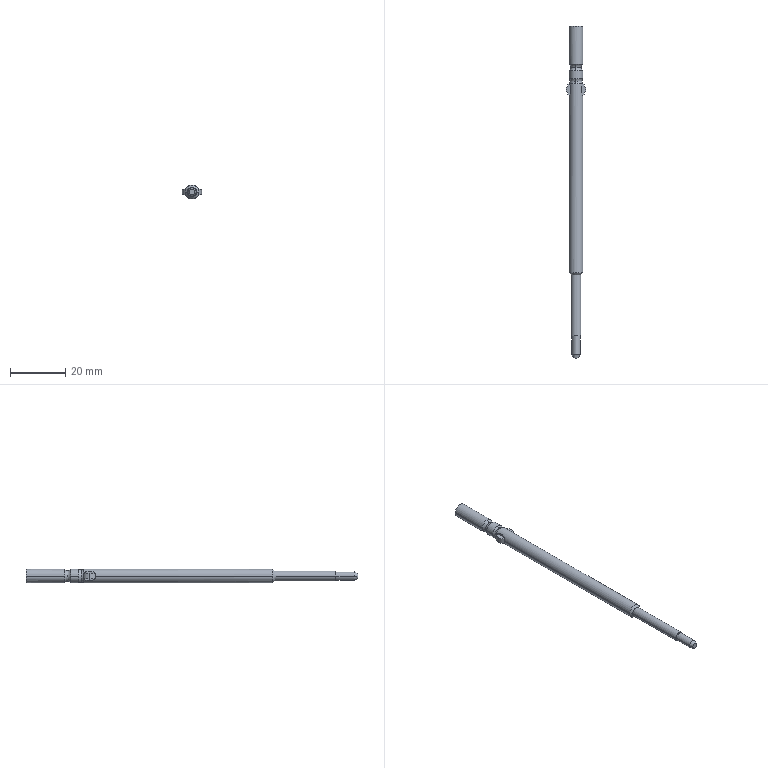Part | SolidWorks | features MoveFace 6, ICE 4, Chamfer 1, MirrorPattern 1, RevCut 1, Revolution 1 | 1 solid | 46 faces | box 7 x 120 x 5 mm | volume 2019 mm3 | cylinder 19 | plane 15 | torus 8 | cone 4 | commonest cylinder face diameters 5 x6 9.339 x6 5.269 x3 2.983 x2 3.5 x2
STEP:
#1=CARTESIAN_POINT('',(0.,116.2,2.5));
#2=VERTEX_POINT('',#1);
#3=CARTESIAN_POINT('',(0.,115.,1.9));
#4=VERTEX_POINT('',#3);
#5=CARTESIAN_POINT('',(0.,115.,3.4));
#6=DIRECTION('',(-1.,0.,0.));
#7=DIRECTION('',(0.,0.,1.));
#8=AXIS2_PLACEMENT_3D('',#5,#6,#7);
#9=CIRCLE('',#8,1.5);
#10=EDGE_CURVE('',#2,#4,#9,.T.);
#11=ORIENTED_EDGE('',*,*,#10,.T.);
#12=CARTESIAN_POINT('',(0.,115.,-1.9));
#13=VERTEX_POINT('',#12);
#14=CARTESIAN_POINT('',(0.,115.,0.));
#15=DIRECTION('',(0.,1.,0.));
#16=DIRECTION('',(0.,0.,1.));
#17=AXIS2_PLACEMENT_3D('',#14,#15,#16);
#18=CIRCLE('',#17,1.9);
#19=EDGE_CURVE('',#4,#13,#18,.T.);
#20=ORIENTED_EDGE('',*,*,#19,.T.);
#21=CARTESIAN_POINT('',(0.,116.2,-2.5));
#22=VERTEX_POINT('',#21);
#23=CARTESIAN_POINT('',(0.,115.,-3.4));
#24=DIRECTION('',(1.,0.,0.));
#25=DIRECTION('',(0.,0.,-1.));
#26=AXIS2_PLACEMENT_3D('',#23,#24,#25);
#27=CIRCLE('',#26,1.5);
#28=EDGE_CURVE('',#22,#13,#27,.T.);
#29=ORIENTED_EDGE('',*,*,#28,.F.);
#30=CARTESIAN_POINT('',(2.5,116.2,0.));
#31=VERTEX_POINT('',#30);
#32=CARTESIAN_POINT('',(0.,116.2,0.));
#33=DIRECTION('',(0.,-1.,0.));
#34=DIRECTION('',(0.,0.,-1.));
#35=AXIS2_PLACEMENT_3D('',#32,#33,#34);
#36=CIRCLE('',#35,2.5);
#37=EDGE_CURVE('',#22,#31,#36,.T.);
#38=ORIENTED_EDGE('',*,*,#37,.T.);
#39=CARTESIAN_POINT('',(0.,116.2,0.));
#40=DIRECTION('',(0.,-1.,0.));
#41=DIRECTION('',(0.,0.,-1.));
#42=AXIS2_PLACEMENT_3D('',#39,#40,#41);
#43=CIRCLE('',#42,2.5);
#44=EDGE_CURVE('',#31,#2,#43,.T.);
#45=ORIENTED_EDGE('',*,*,#44,.T.);
#46=EDGE_LOOP('',(#11,#20,#29,#38,#45));
#47=FACE_OUTER_BOUND('',#46,.T.);
#48=CARTESIAN_POINT('',(0.,115.,0.));
#49=DIRECTION('',(0.,1.,0.));
#50=DIRECTION('',(0.,0.,1.));
#51=AXIS2_PLACEMENT_3D('',#48,#49,#50);
#52=TOROIDAL_SURFACE('',#51,3.4,1.5);
#53=ADVANCED_FACE('',(#47),#52,.F.);
#54=CARTESIAN_POINT('',(0.,110.867,2.5));
#55=VERTEX_POINT('',#54);
#56=CARTESIAN_POINT('',(0.,110.,2.15));
#57=VERTEX_POINT('',#56);
#58=CARTESIAN_POINT('',(0.,110.,3.4));
#59=DIRECTION('',(-1.,0.,0.));
#60=DIRECTION('',(0.,0.,1.));
#61=AXIS2_PLACEMENT_3D('',#58,#59,#60);
#62=CIRCLE('',#61,1.25);
#63=EDGE_CURVE('',#55,#57,#62,.T.);
#64=ORIENTED_EDGE('',*,*,#63,.T.);
#65=CARTESIAN_POINT('',(0.,110.,-2.15));
#66=VERTEX_POINT('',#65);
#67=CARTESIAN_POINT('',(0.,110.,0.));
#68=DIRECTION('',(0.,1.,0.));
#69=DIRECTION('',(0.,0.,1.));
#70=AXIS2_PLACEMENT_3D('',#67,#68,#69);
#71=CIRCLE('',#70,2.15);
#72=EDGE_CURVE('',#57,#66,#71,.T.);
#73=ORIENTED_EDGE('',*,*,#72,.T.);
#74=CARTESIAN_POINT('',(0.,110.867,-2.5));
#75=VERTEX_POINT('',#74);
#76=CARTESIAN_POINT('',(0.,110.,-3.4));
#77=DIRECTION('',(1.,0.,0.));
#78=DIRECTION('',(0.,0.,-1.));
#79=AXIS2_PLACEMENT_3D('',#76,#77,#78);
#80=CIRCLE('',#79,1.25);
#81=EDGE_CURVE('',#75,#66,#80,.T.);
#82=ORIENTED_EDGE('',*,*,#81,.F.);
#83=CARTESIAN_POINT('',(2.5,110.867,0.));
#84=VERTEX_POINT('',#83);
#85=CARTESIAN_POINT('',(0.,110.867,0.));
#86=DIRECTION('',(0.,-1.,0.));
#87=DIRECTION('',(0.,0.,-1.));
#88=AXIS2_PLACEMENT_3D('',#85,#86,#87);
#89=CIRCLE('',#88,2.5);
#90=EDGE_CURVE('',#75,#84,#89,.T.);
#91=ORIENTED_EDGE('',*,*,#90,.T.);
#92=CARTESIAN_POINT('',(0.,110.867,0.));
#93=DIRECTION('',(0.,-1.,0.));
#94=DIRECTION('',(0.,0.,-1.));
#95=AXIS2_PLACEMENT_3D('',#92,#93,#94);
#96=CIRCLE('',#95,2.5);
#97=EDGE_CURVE('',#84,#55,#96,.T.);
#98=ORIENTED_EDGE('',*,*,#97,.T.);
#99=EDGE_LOOP('',(#64,#73,#82,#91,#98));
#100=FACE_OUTER_BOUND('',#99,.T.);
#101=CARTESIAN_POINT('',(0.,110.,0.));
#102=DIRECTION('',(0.,1.,0.));
#103=DIRECTION('',(0.,0.,1.));
#104=AXIS2_PLACEMENT_3D('',#101,#102,#103);
#105=TOROIDAL_SURFACE('',#104,3.4,1.25);
#106=ADVANCED_FACE('',(#100),#105,.F.);
#107=ORIENTED_EDGE('',*,*,#81,.T.);
#108=CARTESIAN_POINT('',(0.,110.,0.));
#109=DIRECTION('',(0.,1.,0.));
#110=DIRECTION('',(0.,0.,1.));
#111=AXIS2_PLACEMENT_3D('',#108,#109,#110);
#112=CIRCLE('',#111,2.15);
#113=EDGE_CURVE('',#66,#57,#112,.T.);
#114=ORIENTED_EDGE('',*,*,#113,.T.);
#115=ORIENTED_EDGE('',*,*,#63,.F.);
#116=CARTESIAN_POINT('',(-2.5,110.867,0.));
#117=VERTEX_POINT('',#116);
#118=CARTESIAN_POINT('',(0.,110.867,0.));
#119=DIRECTION('',(0.,-1.,0.));
#120=DIRECTION('',(0.,0.,-1.));
#121=AXIS2_PLACEMENT_3D('',#118,#119,#120);
#122=CIRCLE('',#121,2.5);
#123=EDGE_CURVE('',#55,#117,#122,.T.);
#124=ORIENTED_EDGE('',*,*,#123,.T.);
#125=CARTESIAN_POINT('',(0.,110.867,0.));
#126=DIRECTION('',(0.,-1.,0.));
#127=DIRECTION('',(0.,0.,-1.));
#128=AXIS2_PLACEMENT_3D('',#125,#126,#127);
#129=CIRCLE('',#128,2.5);
#130=EDGE_CURVE('',#117,#75,#129,.T.);
#131=ORIENTED_EDGE('',*,*,#130,.T.);
#132=EDGE_LOOP('',(#107,#114,#115,#124,#131));
#133=FACE_OUTER_BOUND('',#132,.T.);
#134=CARTESIAN_POINT('',(0.,110.,0.));
#135=DIRECTION('',(0.,1.,0.));
#136=DIRECTION('',(0.,0.,1.));
#137=AXIS2_PLACEMENT_3D('',#134,#135,#136);
#138=TOROIDAL_SURFACE('',#137,3.4,1.25);
#139=ADVANCED_FACE('',(#133),#138,.F.);
#140=ORIENTED_EDGE('',*,*,#28,.T.);
#141=CARTESIAN_POINT('',(0.,115.,0.));
#142=DIRECTION('',(0.,1.,0.));
#143=DIRECTION('',(0.,0.,1.));
#144=AXIS2_PLACEMENT_3D('',#141,#142,#143);
#145=CIRCLE('',#144,1.9);
#146=EDGE_CURVE('',#13,#4,#145,.T.);
#147=ORIENTED_EDGE('',*,*,#146,.T.);
#148=ORIENTED_EDGE('',*,*,#10,.F.);
#149=CARTESIAN_POINT('',(-2.5,116.2,0.));
#150=VERTEX_POINT('',#149);
#151=CARTESIAN_POINT('',(0.,116.2,0.));
#152=DIRECTION('',(0.,-1.,0.));
#153=DIRECTION('',(0.,0.,-1.));
#154=AXIS2_PLACEMENT_3D('',#151,#152,#153);
#155=CIRCLE('',#154,2.5);
#156=EDGE_CURVE('',#2,#150,#155,.T.);
#157=ORIENTED_EDGE('',*,*,#156,.T.);
#158=CARTESIAN_POINT('',(0.,116.2,0.));
#159=DIRECTION('',(0.,-1.,0.));
#160=DIRECTION('',(0.,0.,-1.));
#161=AXIS2_PLACEMENT_3D('',#158,#159,#160);
#162=CIRCLE('',#161,2.5);
#163=EDGE_CURVE('',#150,#22,#162,.T.);
#164=ORIENTED_EDGE('',*,*,#163,.T.);
#165=EDGE_LOOP('',(#140,#147,#148,#157,#164));
#166=FACE_OUTER_BOUND('',#165,.T.);
#167=CARTESIAN_POINT('',(0.,115.,0.));
#168=DIRECTION('',(0.,1.,0.));
#169=DIRECTION('',(0.,0.,1.));
#170=AXIS2_PLACEMENT_3D('',#167,#168,#169);
#171=TOROIDAL_SURFACE('',#170,3.4,1.5);
#172=ADVANCED_FACE('',(#166),#171,.F.);
#173=CARTESIAN_POINT('',(-1.75,40.,0.));
#174=VERTEX_POINT('',#173);
#175=CARTESIAN_POINT('',(1.75,40.,0.));
#176=VERTEX_POINT('',#175);
#177=CARTESIAN_POINT('',(0.,40.,0.));
#178=DIRECTION('',(0.,1.,0.));
#179=DIRECTION('',(-1.,0.,0.));
#180=AXIS2_PLACEMENT_3D('',#177,#178,#179);
#181=CIRCLE('',#180,1.75);
#182=EDGE_CURVE('',#174,#176,#181,.T.);
#183=ORIENTED_EDGE('',*,*,#182,.T.);
#184=CARTESIAN_POINT('',(2.5,40.75,0.));
#185=VERTEX_POINT('',#184);
#186=CARTESIAN_POINT('',(2.5,40.75,0.));
#187=DIRECTION('',(0.7071,0.7071,0.));
#188=VECTOR('',#187,1000.);
#189=LINE('',#186,#188);
#190=EDGE_CURVE('',#176,#185,#189,.T.);
#191=ORIENTED_EDGE('',*,*,#190,.T.);
#192=CARTESIAN_POINT('',(-2.5,40.75,0.));
#193=VERTEX_POINT('',#192);
#194=CARTESIAN_POINT('',(0.,40.75,0.));
#195=DIRECTION('',(0.,1.,0.));
#196=DIRECTION('',(-1.,0.,0.));
#197=AXIS2_PLACEMENT_3D('',#194,#195,#196);
#198=CIRCLE('',#197,2.5);
#199=EDGE_CURVE('',#193,#185,#198,.T.);
#200=ORIENTED_EDGE('',*,*,#199,.F.);
#201=CARTESIAN_POINT('',(-2.5,40.75,0.));
#202=DIRECTION('',(-0.7071,0.7071,0.));
#203=VECTOR('',#202,1000.);
#204=LINE('',#201,#203);
#205=EDGE_CURVE('',#174,#193,#204,.T.);
#206=ORIENTED_EDGE('',*,*,#205,.F.);
#207=EDGE_LOOP('',(#183,#191,#200,#206));
#208=FACE_OUTER_BOUND('',#207,.T.);
#209=CARTESIAN_POINT('',(0.,40.75,0.));
#210=DIRECTION('',(0.,1.,0.));
#211=DIRECTION('',(-1.,0.,0.));
#212=AXIS2_PLACEMENT_3D('',#209,#210,#211);
#213=CONICAL_SURFACE('',#212,2.5,0.7854);
#214=ADVANCED_FACE('',(#208),#213,.T.);
#215=CARTESIAN_POINT('',(-1.017,10.,0.));
#216=VERTEX_POINT('',#215);
#217=CARTESIAN_POINT('',(1.017,10.,0.));
#218=VERTEX_POINT('',#217);
#219=CARTESIAN_POINT('',(0.,10.,0.));
#220=DIRECTION('',(0.,1.,0.));
#221=DIRECTION('',(-1.,0.,0.));
#222=AXIS2_PLACEMENT_3D('',#219,#220,#221);
#223=CIRCLE('',#222,1.017);
#224=EDGE_CURVE('',#216,#218,#223,.T.);
#225=ORIENTED_EDGE('',*,*,#224,.T.);
#226=CARTESIAN_POINT('',(1.491,11.265,0.));
#227=VERTEX_POINT('',#226);
#228=CARTESIAN_POINT('',(0.9841,9.912,0.));
#229=DIRECTION('',(0.3511,0.9363,0.));
#230=VECTOR('',#229,1000.);
#231=LINE('',#228,#230);
#232=EDGE_CURVE('',#218,#227,#231,.T.);
#233=ORIENTED_EDGE('',*,*,#232,.T.);
#234=CARTESIAN_POINT('',(-1.491,11.265,0.));
#235=VERTEX_POINT('',#234);
#236=CARTESIAN_POINT('',(0.,11.265,0.));
#237=DIRECTION('',(0.,1.,0.));
#238=DIRECTION('',(-1.,0.,0.));
#239=AXIS2_PLACEMENT_3D('',#236,#237,#238);
#240=CIRCLE('',#239,1.491);
#241=EDGE_CURVE('',#235,#227,#240,.T.);
#242=ORIENTED_EDGE('',*,*,#241,.F.);
#243=CARTESIAN_POINT('',(-0.9841,9.912,0.));
#244=DIRECTION('',(-0.3511,0.9363,0.));
#245=VECTOR('',#244,1000.);
#246=LINE('',#243,#245);
#247=EDGE_CURVE('',#216,#235,#246,.T.);
#248=ORIENTED_EDGE('',*,*,#247,.F.);
#249=EDGE_LOOP('',(#225,#233,#242,#248));
#250=FACE_OUTER_BOUND('',#249,.T.);
#251=CARTESIAN_POINT('',(0.,9.912,0.));
#252=DIRECTION('',(0.,1.,0.));
#253=DIRECTION('',(-1.,0.,0.));
#254=AXIS2_PLACEMENT_3D('',#251,#252,#253);
#255=CONICAL_SURFACE('',#254,0.9841,0.3588);
#256=ADVANCED_FACE('',(#250),#255,.T.);
#257=CARTESIAN_POINT('',(1.491,18.,0.));
#258=VERTEX_POINT('',#257);
#259=CARTESIAN_POINT('',(-1.491,18.,0.));
#260=VERTEX_POINT('',#259);
#261=CARTESIAN_POINT('',(0.,18.,0.));
#262=DIRECTION('',(0.,-1.,0.));
#263=DIRECTION('',(1.,0.,0.));
#264=AXIS2_PLACEMENT_3D('',#261,#262,#263);
#265=CIRCLE('',#264,1.491);
#266=EDGE_CURVE('',#258,#260,#265,.T.);
#267=ORIENTED_EDGE('',*,*,#266,.T.);
#268=CARTESIAN_POINT('',(-1.491,8.,0.));
#269=DIRECTION('',(0.,-1.,0.));
#270=VECTOR('',#269,1000.);
#271=LINE('',#268,#270);
#272=EDGE_CURVE('',#260,#235,#271,.T.);
#273=ORIENTED_EDGE('',*,*,#272,.T.);
#274=ORIENTED_EDGE('',*,*,#241,.T.);
#275=CARTESIAN_POINT('',(1.491,8.,0.));
#276=DIRECTION('',(0.,-1.,0.));
#277=VECTOR('',#276,1000.);
#278=LINE('',#275,#277);
#279=EDGE_CURVE('',#258,#227,#278,.T.);
#280=ORIENTED_EDGE('',*,*,#279,.F.);
#281=EDGE_LOOP('',(#267,#273,#274,#280));
#282=FACE_OUTER_BOUND('',#281,.T.);
#283=CARTESIAN_POINT('',(0.,8.,0.));
#284=DIRECTION('',(0.,-1.,0.));
#285=DIRECTION('',(1.,0.,0.));
#286=AXIS2_PLACEMENT_3D('',#283,#284,#285);
#287=CYLINDRICAL_SURFACE('',#286,1.491);
#288=ADVANCED_FACE('',(#282),#287,.T.);
#289=CARTESIAN_POINT('',(-1.809,107.066,-1.725));
#290=VERTEX_POINT('',#289);
#291=CARTESIAN_POINT('',(-2.291,109.133,-1.));
#292=VERTEX_POINT('',#291);
#293=CARTESIAN_POINT('',(-1.809,107.066,-1.725));
#294=CARTESIAN_POINT('',(-1.809,107.454,-1.725));
#295=CARTESIAN_POINT('',(-1.858,107.835,-1.679));
#296=CARTESIAN_POINT('',(-1.993,108.376,-1.511));
#297=CARTESIAN_POINT('',(-2.047,108.547,-1.44));
#298=CARTESIAN_POINT('',(-2.166,108.864,-1.254));
#299=CARTESIAN_POINT('',(-2.231,109.01,-1.139));
#300=CARTESIAN_POINT('',(-2.291,109.133,-1.));
#301=B_SPLINE_CURVE_WITH_KNOTS('',3,(#293,#294,#295,#296,#297,#298,#299,#300),.UNSPECIFIED.,.F.,.F.,(4,2,2,4),(0.01141,0.01257,0.01314,0.01372),.UNSPECIFIED.);
#302=EDGE_CURVE('',#290,#292,#301,.T.);
#303=ORIENTED_EDGE('',*,*,#302,.F.);
#304=CARTESIAN_POINT('',(-1.809,107.066,-1.));
#305=VERTEX_POINT('',#304);
#306=CARTESIAN_POINT('',(-1.809,107.066,-4.));
#307=DIRECTION('',(0.,0.,1.));
#308=VECTOR('',#307,1000.);
#309=LINE('',#306,#308);
#310=EDGE_CURVE('',#290,#305,#309,.T.);
#311=ORIENTED_EDGE('',*,*,#310,.T.);
#312=CARTESIAN_POINT('',(-6.479,107.066,-1.));
#313=DIRECTION('',(0.,0.,1.));
#314=DIRECTION('',(-1.,0.,0.));
#315=AXIS2_PLACEMENT_3D('',#312,#313,#314);
#316=CIRCLE('',#315,4.669);
#317=EDGE_CURVE('',#305,#292,#316,.T.);
#318=ORIENTED_EDGE('',*,*,#317,.T.);
#319=EDGE_LOOP('',(#303,#311,#318));
#320=FACE_OUTER_BOUND('',#319,.T.);
#321=CARTESIAN_POINT('',(-6.479,107.066,-4.));
#322=DIRECTION('',(0.,0.,1.));
#323=DIRECTION('',(1.,0.,0.));
#324=AXIS2_PLACEMENT_3D('',#321,#322,#323);
#325=CYLINDRICAL_SURFACE('',#324,4.669);
#326=ADVANCED_FACE('',(#320),#325,.F.);
#327=CARTESIAN_POINT('',(2.291,109.133,1.));
#328=VERTEX_POINT('',#327);
#329=CARTESIAN_POINT('',(1.809,107.066,1.725));
#330=VERTEX_POINT('',#329);
#331=CARTESIAN_POINT('',(2.291,109.133,1.));
#332=CARTESIAN_POINT('',(2.231,109.009,1.139));
#333=CARTESIAN_POINT('',(2.167,108.867,1.252));
#334=CARTESIAN_POINT('',(2.047,108.548,1.439));
#335=CARTESIAN_POINT('',(1.993,108.377,1.511));
#336=CARTESIAN_POINT('',(1.904,108.02,1.622));
#337=CARTESIAN_POINT('',(1.868,107.831,1.661));
#338=CARTESIAN_POINT('',(1.821,107.452,1.713));
#339=CARTESIAN_POINT('',(1.809,107.26,1.725));
#340=CARTESIAN_POINT('',(1.809,107.066,1.725));
#341=B_SPLINE_CURVE_WITH_KNOTS('',3,(#331,#332,#333,#334,#335,#336,#337,#338,#339,#340),.UNSPECIFIED.,.F.,.F.,(4,2,2,2,4),(0.009093,0.009672,0.01025,0.01083,0.01141),.UNSPECIFIED.);
#342=EDGE_CURVE('',#328,#330,#341,.T.);
#343=ORIENTED_EDGE('',*,*,#342,.T.);
#344=CARTESIAN_POINT('',(1.809,107.066,1.));
#345=VERTEX_POINT('',#344);
#346=CARTESIAN_POINT('',(1.809,107.066,4.));
#347=DIRECTION('',(0.,0.,-1.));
#348=VECTOR('',#347,1000.);
#349=LINE('',#346,#348);
#350=EDGE_CURVE('',#330,#345,#349,.T.);
#351=ORIENTED_EDGE('',*,*,#350,.T.);
#352=CARTESIAN_POINT('',(6.479,107.066,1.));
#353=DIRECTION('',(0.,0.,1.));
#354=DIRECTION('',(1.,0.,0.));
#355=AXIS2_PLACEMENT_3D('',#352,#353,#354);
#356=CIRCLE('',#355,4.669);
#357=EDGE_CURVE('',#328,#345,#356,.T.);
#358=ORIENTED_EDGE('',*,*,#357,.F.);
#359=EDGE_LOOP('',(#343,#351,#358));
#360=FACE_OUTER_BOUND('',#359,.T.);
#361=CARTESIAN_POINT('',(6.479,107.066,4.));
#362=DIRECTION('',(0.,0.,-1.));
#363=DIRECTION('',(-1.,0.,0.));
#364=AXIS2_PLACEMENT_3D('',#361,#362,#363);
#365=CYLINDRICAL_SURFACE('',#364,4.669);
#366=ADVANCED_FACE('',(#360),#365,.F.);
#367=CARTESIAN_POINT('',(-3.5,107.066,1.));
#368=VERTEX_POINT('',#367);
#369=CARTESIAN_POINT('',(-2.5,105.,1.));
#370=VERTEX_POINT('',#369);
#371=CARTESIAN_POINT('',(-0.8653,107.066,1.));
#372=DIRECTION('',(0.,0.,1.));
#373=DIRECTION('',(1.,0.,0.));
#374=AXIS2_PLACEMENT_3D('',#371,#372,#373);
#375=CIRCLE('',#374,2.635);
#376=EDGE_CURVE('',#368,#370,#375,.T.);
#377=ORIENTED_EDGE('',*,*,#376,.F.);
#378=CARTESIAN_POINT('',(-3.5,107.066,-1.));
#379=VERTEX_POINT('',#378);
#380=CARTESIAN_POINT('',(-3.5,107.066,1.));
#381=DIRECTION('',(0.,0.,-1.));
#382=VECTOR('',#381,1000.);
#383=LINE('',#380,#382);
#384=EDGE_CURVE('',#368,#379,#383,.T.);
#385=ORIENTED_EDGE('',*,*,#384,.T.);
#386=CARTESIAN_POINT('',(-2.5,105.,-1.));
#387=VERTEX_POINT('',#386);
#388=CARTESIAN_POINT('',(-0.8653,107.066,-1.));
#389=DIRECTION('',(0.,0.,1.));
#390=DIRECTION('',(1.,0.,0.));
#391=AXIS2_PLACEMENT_3D('',#388,#389,#390);
#392=CIRCLE('',#391,2.635);
#393=EDGE_CURVE('',#379,#387,#392,.T.);
#394=ORIENTED_EDGE('',*,*,#393,.T.);
#395=CARTESIAN_POINT('',(-2.5,105.,0.));
#396=VERTEX_POINT('',#395);
#397=CARTESIAN_POINT('',(-2.5,105.,1.));
#398=DIRECTION('',(0.,0.,-1.));
#399=VECTOR('',#398,1000.);
#400=LINE('',#397,#399);
#401=EDGE_CURVE('',#396,#387,#400,.T.);
#402=ORIENTED_EDGE('',*,*,#401,.F.);
#403=CARTESIAN_POINT('',(-2.5,105.,1.));
#404=DIRECTION('',(0.,0.,-1.));
#405=VECTOR('',#404,1000.);
#406=LINE('',#403,#405);
#407=EDGE_CURVE('',#370,#396,#406,.T.);
#408=ORIENTED_EDGE('',*,*,#407,.F.);
#409=EDGE_LOOP('',(#377,#385,#394,#402,#408));
#410=FACE_OUTER_BOUND('',#409,.T.);
#411=CARTESIAN_POINT('',(-0.8653,107.066,1.));
#412=DIRECTION('',(0.,0.,-1.));
#413=DIRECTION('',(-1.,0.,0.));
#414=AXIS2_PLACEMENT_3D('',#411,#412,#413);
#415=CYLINDRICAL_SURFACE('',#414,2.635);
#416=ADVANCED_FACE('',(#410),#415,.T.);
#417=ORIENTED_EDGE('',*,*,#97,.F.);
#418=CARTESIAN_POINT('',(2.5,113.8,0.));
#419=VERTEX_POINT('',#418);
#420=CARTESIAN_POINT('',(2.5,120.,0.));
#421=DIRECTION('',(0.,1.,0.));
#422=VECTOR('',#421,1000.);
#423=LINE('',#420,#422);
#424=EDGE_CURVE('',#84,#419,#423,.T.);
#425=ORIENTED_EDGE('',*,*,#424,.T.);
#426=CARTESIAN_POINT('',(0.,113.8,2.5));
#427=VERTEX_POINT('',#426);
#428=CARTESIAN_POINT('',(0.,113.8,0.));
#429=DIRECTION('',(0.,1.,0.));
#430=DIRECTION('',(0.,0.,1.));
#431=AXIS2_PLACEMENT_3D('',#428,#429,#430);
#432=CIRCLE('',#431,2.5);
#433=EDGE_CURVE('',#427,#419,#432,.T.);
#434=ORIENTED_EDGE('',*,*,#433,.F.);
#435=CARTESIAN_POINT('',(-2.5,113.8,0.));
#436=VERTEX_POINT('',#435);
#437=CARTESIAN_POINT('',(0.,113.8,0.));
#438=DIRECTION('',(0.,1.,0.));
#439=DIRECTION('',(0.,0.,1.));
#440=AXIS2_PLACEMENT_3D('',#437,#438,#439);
#441=CIRCLE('',#440,2.5);
#442=EDGE_CURVE('',#436,#427,#441,.T.);
#443=ORIENTED_EDGE('',*,*,#442,.F.);
#444=CARTESIAN_POINT('',(-2.5,120.,0.));
#445=DIRECTION('',(0.,1.,0.));
#446=VECTOR('',#445,1000.);
#447=LINE('',#444,#446);
#448=EDGE_CURVE('',#117,#436,#447,.T.);
#449=ORIENTED_EDGE('',*,*,#448,.F.);
#450=ORIENTED_EDGE('',*,*,#123,.F.);
#451=EDGE_LOOP('',(#417,#425,#434,#443,#449,#450));
#452=FACE_OUTER_BOUND('',#451,.T.);
#453=CARTESIAN_POINT('',(0.,120.,0.));
#454=DIRECTION('',(0.,1.,0.));
#455=DIRECTION('',(-1.,0.,0.));
#456=AXIS2_PLACEMENT_3D('',#453,#454,#455);
#457=CYLINDRICAL_SURFACE('',#456,2.5);
#458=ADVANCED_FACE('',(#452),#457,.T.);
#459=ORIENTED_EDGE('',*,*,#146,.F.);
#460=CARTESIAN_POINT('',(0.,113.8,-2.5));
#461=VERTEX_POINT('',#460);
#462=CARTESIAN_POINT('',(0.,115.,-3.4));
#463=DIRECTION('',(1.,0.,0.));
#464=DIRECTION('',(0.,0.,-1.));
#465=AXIS2_PLACEMENT_3D('',#462,#463,#464);
#466=CIRCLE('',#465,1.5);
#467=EDGE_CURVE('',#13,#461,#466,.T.);
#468=ORIENTED_EDGE('',*,*,#467,.T.);
#469=CARTESIAN_POINT('',(0.,113.8,0.));
#470=DIRECTION('',(0.,1.,0.));
#471=DIRECTION('',(0.,0.,1.));
#472=AXIS2_PLACEMENT_3D('',#469,#470,#471);
#473=CIRCLE('',#472,2.5);
#474=EDGE_CURVE('',#461,#436,#473,.T.);
#475=ORIENTED_EDGE('',*,*,#474,.T.);
#476=ORIENTED_EDGE('',*,*,#442,.T.);
#477=CARTESIAN_POINT('',(0.,115.,3.4));
#478=DIRECTION('',(-1.,0.,0.));
#479=DIRECTION('',(0.,0.,1.));
#480=AXIS2_PLACEMENT_3D('',#477,#478,#479);
#481=CIRCLE('',#480,1.5);
#482=EDGE_CURVE('',#4,#427,#481,.T.);
#483=ORIENTED_EDGE('',*,*,#482,.F.);
#484=EDGE_LOOP('',(#459,#468,#475,#476,#483));
#485=FACE_OUTER_BOUND('',#484,.T.);
#486=CARTESIAN_POINT('',(0.,115.,0.));
#487=DIRECTION('',(0.,1.,0.));
#488=DIRECTION('',(0.,0.,1.));
#489=AXIS2_PLACEMENT_3D('',#486,#487,#488);
#490=TOROIDAL_SURFACE('',#489,3.4,1.5);
#491=ADVANCED_FACE('',(#485),#490,.F.);
#492=ORIENTED_EDGE('',*,*,#44,.F.);
#493=CARTESIAN_POINT('',(2.5,130.,0.));
#494=VERTEX_POINT('',#493);
#495=CARTESIAN_POINT('',(2.5,120.,0.));
#496=DIRECTION('',(0.,1.,0.));
#497=VECTOR('',#496,1000.);
#498=LINE('',#495,#497);
#499=EDGE_CURVE('',#31,#494,#498,.T.);
#500=ORIENTED_EDGE('',*,*,#499,.T.);
#501=CARTESIAN_POINT('',(-2.5,130.,0.));
#502=VERTEX_POINT('',#501);
#503=CARTESIAN_POINT('',(0.,130.,0.));
#504=DIRECTION('',(0.,1.,0.));
#505=DIRECTION('',(-1.,0.,0.));
#506=AXIS2_PLACEMENT_3D('',#503,#504,#505);
#507=CIRCLE('',#506,2.5);
#508=EDGE_CURVE('',#502,#494,#507,.T.);
#509=ORIENTED_EDGE('',*,*,#508,.F.);
#510=CARTESIAN_POINT('',(-2.5,120.,0.));
#511=DIRECTION('',(0.,1.,0.));
#512=VECTOR('',#511,1000.);
#513=LINE('',#510,#512);
#514=EDGE_CURVE('',#150,#502,#513,.T.);
#515=ORIENTED_EDGE('',*,*,#514,.F.);
#516=ORIENTED_EDGE('',*,*,#156,.F.);
#517=EDGE_LOOP('',(#492,#500,#509,#515,#516));
#518=FACE_OUTER_BOUND('',#517,.T.);
#519=CARTESIAN_POINT('',(0.,120.,0.));
#520=DIRECTION('',(0.,1.,0.));
#521=DIRECTION('',(-1.,0.,0.));
#522=AXIS2_PLACEMENT_3D('',#519,#520,#521);
#523=CYLINDRICAL_SURFACE('',#522,2.5);
#524=ADVANCED_FACE('',(#518),#523,.T.);
#525=ORIENTED_EDGE('',*,*,#113,.F.);
#526=CARTESIAN_POINT('',(0.,109.133,-2.5));
#527=VERTEX_POINT('',#526);
#528=CARTESIAN_POINT('',(0.,110.,-3.4));
#529=DIRECTION('',(1.,0.,0.));
#530=DIRECTION('',(0.,0.,-1.));
#531=AXIS2_PLACEMENT_3D('',#528,#529,#530);
#532=CIRCLE('',#531,1.25);
#533=EDGE_CURVE('',#66,#527,#532,.T.);
#534=ORIENTED_EDGE('',*,*,#533,.T.);
#535=CARTESIAN_POINT('',(0.,109.133,0.));
#536=DIRECTION('',(0.,1.,0.));
#537=DIRECTION('',(0.,0.,1.));
#538=AXIS2_PLACEMENT_3D('',#535,#536,#537);
#539=CIRCLE('',#538,2.5);
#540=EDGE_CURVE('',#527,#292,#539,.T.);
#541=ORIENTED_EDGE('',*,*,#540,.T.);
#542=CARTESIAN_POINT('',(-2.5,109.133,0.));
#543=VERTEX_POINT('',#542);
#544=CARTESIAN_POINT('',(0.,109.133,0.));
#545=DIRECTION('',(0.,1.,0.));
#546=DIRECTION('',(0.,0.,1.));
#547=AXIS2_PLACEMENT_3D('',#544,#545,#546);
#548=CIRCLE('',#547,2.5);
#549=EDGE_CURVE('',#292,#543,#548,.T.);
#550=ORIENTED_EDGE('',*,*,#549,.T.);
#551=CARTESIAN_POINT('',(-2.291,109.133,1.));
#552=VERTEX_POINT('',#551);
#553=CARTESIAN_POINT('',(0.,109.133,0.));
#554=DIRECTION('',(0.,1.,0.));
#555=DIRECTION('',(0.,0.,1.));
#556=AXIS2_PLACEMENT_3D('',#553,#554,#555);
#557=CIRCLE('',#556,2.5);
#558=EDGE_CURVE('',#543,#552,#557,.T.);
#559=ORIENTED_EDGE('',*,*,#558,.T.);
#560=CARTESIAN_POINT('',(0.,109.133,2.5));
#561=VERTEX_POINT('',#560);
#562=CARTESIAN_POINT('',(0.,109.133,0.));
#563=DIRECTION('',(0.,1.,0.));
#564=DIRECTION('',(0.,0.,1.));
#565=AXIS2_PLACEMENT_3D('',#562,#563,#564);
#566=CIRCLE('',#565,2.5);
#567=EDGE_CURVE('',#552,#561,#566,.T.);
#568=ORIENTED_EDGE('',*,*,#567,.T.);
#569=CARTESIAN_POINT('',(0.,110.,3.4));
#570=DIRECTION('',(-1.,0.,0.));
#571=DIRECTION('',(0.,0.,1.));
#572=AXIS2_PLACEMENT_3D('',#569,#570,#571);
#573=CIRCLE('',#572,1.25);
#574=EDGE_CURVE('',#57,#561,#573,.T.);
#575=ORIENTED_EDGE('',*,*,#574,.F.);
#576=EDGE_LOOP('',(#525,#534,#541,#550,#559,#568,#575));
#577=FACE_OUTER_BOUND('',#576,.T.);
#578=CARTESIAN_POINT('',(0.,110.,0.));
#579=DIRECTION('',(0.,1.,0.));
#580=DIRECTION('',(0.,0.,1.));
#581=AXIS2_PLACEMENT_3D('',#578,#579,#580);
#582=TOROIDAL_SURFACE('',#581,3.4,1.25);
#583=ADVANCED_FACE('',(#577),#582,.F.);
#584=ORIENTED_EDGE('',*,*,#199,.T.);
#585=CARTESIAN_POINT('',(2.5,105.,0.));
#586=VERTEX_POINT('',#585);
#587=CARTESIAN_POINT('',(2.5,120.,0.));
#588=DIRECTION('',(0.,1.,0.));
#589=VECTOR('',#588,1000.);
#590=LINE('',#587,#589);
#591=EDGE_CURVE('',#185,#586,#590,.T.);
#592=ORIENTED_EDGE('',*,*,#591,.T.);
#593=CARTESIAN_POINT('',(2.291,105.,1.));
#594=VERTEX_POINT('',#593);
#595=CARTESIAN_POINT('',(0.,105.,0.));
#596=DIRECTION('',(0.,1.,0.));
#597=DIRECTION('',(0.,0.,1.));
#598=AXIS2_PLACEMENT_3D('',#595,#596,#597);
#599=CIRCLE('',#598,2.5);
#600=EDGE_CURVE('',#594,#586,#599,.T.);
#601=ORIENTED_EDGE('',*,*,#600,.F.);
#602=CARTESIAN_POINT('',(1.809,107.066,1.725));
#603=CARTESIAN_POINT('',(1.809,106.679,1.725));
#604=CARTESIAN_POINT('',(1.858,106.298,1.679));
#605=CARTESIAN_POINT('',(1.993,105.756,1.511));
#606=CARTESIAN_POINT('',(2.047,105.586,1.44));
#607=CARTESIAN_POINT('',(2.166,105.269,1.254));
#608=CARTESIAN_POINT('',(2.231,105.123,1.139));
#609=CARTESIAN_POINT('',(2.291,105.,1.));
#610=B_SPLINE_CURVE_WITH_KNOTS('',3,(#602,#603,#604,#605,#606,#607,#608,#609),.UNSPECIFIED.,.F.,.F.,(4,2,2,4),(0.01141,0.01257,0.01314,0.01372),.UNSPECIFIED.);
#611=EDGE_CURVE('',#330,#594,#610,.T.);
#612=ORIENTED_EDGE('',*,*,#611,.F.);
#613=ORIENTED_EDGE('',*,*,#342,.F.);
#614=CARTESIAN_POINT('',(0.,109.133,0.));
#615=DIRECTION('',(0.,1.,0.));
#616=DIRECTION('',(0.,0.,1.));
#617=AXIS2_PLACEMENT_3D('',#614,#615,#616);
#618=CIRCLE('',#617,2.5);
#619=EDGE_CURVE('',#561,#328,#618,.T.);
#620=ORIENTED_EDGE('',*,*,#619,.F.);
#621=ORIENTED_EDGE('',*,*,#567,.F.);
#622=CARTESIAN_POINT('',(-2.291,105.,1.));
#623=VERTEX_POINT('',#622);
#624=CARTESIAN_POINT('',(-2.291,105.,1.));
#625=CARTESIAN_POINT('',(-2.231,105.123,1.139));
#626=CARTESIAN_POINT('',(-2.167,105.266,1.252));
#627=CARTESIAN_POINT('',(-2.047,105.584,1.439));
#628=CARTESIAN_POINT('',(-1.993,105.756,1.511));
#629=CARTESIAN_POINT('',(-1.904,106.113,1.622));
#630=CARTESIAN_POINT('',(-1.868,106.301,1.661));
#631=CARTESIAN_POINT('',(-1.821,106.68,1.713));
#632=CARTESIAN_POINT('',(-1.809,106.872,1.725));
#633=CARTESIAN_POINT('',(-1.809,107.454,1.725));
#634=CARTESIAN_POINT('',(-1.858,107.834,1.679));
#635=CARTESIAN_POINT('',(-1.993,108.376,1.511));
#636=CARTESIAN_POINT('',(-2.047,108.547,1.44));
#637=CARTESIAN_POINT('',(-2.166,108.864,1.254));
#638=CARTESIAN_POINT('',(-2.231,109.01,1.139));
#639=CARTESIAN_POINT('',(-2.291,109.133,1.));
#640=B_SPLINE_CURVE_WITH_KNOTS('',3,(#624,#625,#626,#627,#628,#629,#630,#631,#632,#633,#634,#635,#636,#637,#638,#639),.UNSPECIFIED.,.F.,.F.,(4,2,2,2,2,2,2,4),(0.009093,0.009672,0.01025,0.01083,0.01141,0.01257,0.01314,0.01372),.UNSPECIFIED.);
#641=EDGE_CURVE('',#623,#552,#640,.T.);
#642=ORIENTED_EDGE('',*,*,#641,.F.);
#643=CARTESIAN_POINT('',(0.,105.,0.));
#644=DIRECTION('',(0.,1.,0.));
#645=DIRECTION('',(0.,0.,1.));
#646=AXIS2_PLACEMENT_3D('',#643,#644,#645);
#647=CIRCLE('',#646,2.5);
#648=EDGE_CURVE('',#396,#623,#647,.T.);
#649=ORIENTED_EDGE('',*,*,#648,.F.);
#650=CARTESIAN_POINT('',(-2.5,120.,0.));
#651=DIRECTION('',(0.,1.,0.));
#652=VECTOR('',#651,1000.);
#653=LINE('',#650,#652);
#654=EDGE_CURVE('',#193,#396,#653,.T.);
#655=ORIENTED_EDGE('',*,*,#654,.F.);
#656=EDGE_LOOP('',(#584,#592,#601,#612,#613,#620,#621,#642,#649,#655));
#657=FACE_OUTER_BOUND('',#656,.T.);
#658=CARTESIAN_POINT('',(0.,120.,0.));
#659=DIRECTION('',(0.,1.,0.));
#660=DIRECTION('',(-1.,0.,0.));
#661=AXIS2_PLACEMENT_3D('',#658,#659,#660);
#662=CYLINDRICAL_SURFACE('',#661,2.5);
#663=ADVANCED_FACE('',(#657),#662,.T.);
#664=CARTESIAN_POINT('',(1.75,18.,0.));
#665=VERTEX_POINT('',#664);
#666=CARTESIAN_POINT('',(-1.75,18.,0.));
#667=VERTEX_POINT('',#666);
#668=CARTESIAN_POINT('',(0.,18.,0.));
#669=DIRECTION('',(0.,-1.,0.));
#670=DIRECTION('',(1.,0.,0.));
#671=AXIS2_PLACEMENT_3D('',#668,#669,#670);
#672=CIRCLE('',#671,1.75);
#673=EDGE_CURVE('',#665,#667,#672,.T.);
#674=ORIENTED_EDGE('',*,*,#673,.F.);
#675=CARTESIAN_POINT('',(1.75,120.,0.));
#676=DIRECTION('',(0.,1.,0.));
#677=VECTOR('',#676,1000.);
#678=LINE('',#675,#677);
#679=EDGE_CURVE('',#665,#176,#678,.T.);
#680=ORIENTED_EDGE('',*,*,#679,.T.);
#681=ORIENTED_EDGE('',*,*,#182,.F.);
#682=CARTESIAN_POINT('',(-1.75,120.,0.));
#683=DIRECTION('',(0.,1.,0.));
#684=VECTOR('',#683,1000.);
#685=LINE('',#682,#684);
#686=EDGE_CURVE('',#667,#174,#685,.T.);
#687=ORIENTED_EDGE('',*,*,#686,.F.);
#688=EDGE_LOOP('',(#674,#680,#681,#687));
#689=FACE_OUTER_BOUND('',#688,.T.);
#690=CARTESIAN_POINT('',(0.,120.,0.));
#691=DIRECTION('',(0.,1.,0.));
#692=DIRECTION('',(-1.,0.,0.));
#693=AXIS2_PLACEMENT_3D('',#690,#691,#692);
#694=CYLINDRICAL_SURFACE('',#693,1.75);
#695=ADVANCED_FACE('',(#689),#694,.T.);
#696=ORIENTED_EDGE('',*,*,#679,.F.);
#697=CARTESIAN_POINT('',(0.,18.,0.));
#698=DIRECTION('',(0.,-1.,0.));
#699=DIRECTION('',(1.,0.,0.));
#700=AXIS2_PLACEMENT_3D('',#697,#698,#699);
#701=CIRCLE('',#700,1.75);
#702=EDGE_CURVE('',#667,#665,#701,.T.);
#703=ORIENTED_EDGE('',*,*,#702,.F.);
#704=ORIENTED_EDGE('',*,*,#686,.T.);
#705=CARTESIAN_POINT('',(0.,40.,0.));
#706=DIRECTION('',(0.,1.,0.));
#707=DIRECTION('',(-1.,0.,0.));
#708=AXIS2_PLACEMENT_3D('',#705,#706,#707);
#709=CIRCLE('',#708,1.75);
#710=EDGE_CURVE('',#176,#174,#709,.T.);
#711=ORIENTED_EDGE('',*,*,#710,.F.);
#712=EDGE_LOOP('',(#696,#703,#704,#711));
#713=FACE_OUTER_BOUND('',#712,.T.);
#714=CARTESIAN_POINT('',(0.,120.,0.));
#715=DIRECTION('',(0.,1.,0.));
#716=DIRECTION('',(-1.,0.,0.));
#717=AXIS2_PLACEMENT_3D('',#714,#715,#716);
#718=CYLINDRICAL_SURFACE('',#717,1.75);
#719=ADVANCED_FACE('',(#713),#718,.T.);
#720=ORIENTED_EDGE('',*,*,#591,.F.);
#721=CARTESIAN_POINT('',(0.,40.75,0.));
#722=DIRECTION('',(0.,1.,0.));
#723=DIRECTION('',(-1.,0.,0.));
#724=AXIS2_PLACEMENT_3D('',#721,#722,#723);
#725=CIRCLE('',#724,2.5);
#726=EDGE_CURVE('',#185,#193,#725,.T.);
#727=ORIENTED_EDGE('',*,*,#726,.T.);
#728=ORIENTED_EDGE('',*,*,#654,.T.);
#729=CARTESIAN_POINT('',(-2.291,105.,-1.));
#730=VERTEX_POINT('',#729);
#731=CARTESIAN_POINT('',(0.,105.,0.));
#732=DIRECTION('',(0.,1.,0.));
#733=DIRECTION('',(0.,0.,1.));
#734=AXIS2_PLACEMENT_3D('',#731,#732,#733);
#735=CIRCLE('',#734,2.5);
#736=EDGE_CURVE('',#730,#396,#735,.T.);
#737=ORIENTED_EDGE('',*,*,#736,.F.);
#738=CARTESIAN_POINT('',(-2.291,105.,-1.));
#739=CARTESIAN_POINT('',(-2.231,105.123,-1.139));
#740=CARTESIAN_POINT('',(-2.167,105.266,-1.252));
#741=CARTESIAN_POINT('',(-2.047,105.584,-1.439));
#742=CARTESIAN_POINT('',(-1.993,105.756,-1.511));
#743=CARTESIAN_POINT('',(-1.904,106.113,-1.622));
#744=CARTESIAN_POINT('',(-1.868,106.301,-1.661));
#745=CARTESIAN_POINT('',(-1.821,106.681,-1.713));
#746=CARTESIAN_POINT('',(-1.809,106.872,-1.725));
#747=CARTESIAN_POINT('',(-1.809,107.066,-1.725));
#748=B_SPLINE_CURVE_WITH_KNOTS('',3,(#738,#739,#740,#741,#742,#743,#744,#745,#746,#747),.UNSPECIFIED.,.F.,.F.,(4,2,2,2,4),(0.009093,0.009672,0.01025,0.01083,0.01141),.UNSPECIFIED.);
#749=EDGE_CURVE('',#730,#290,#748,.T.);
#750=ORIENTED_EDGE('',*,*,#749,.T.);
#751=ORIENTED_EDGE('',*,*,#302,.T.);
#752=ORIENTED_EDGE('',*,*,#540,.F.);
#753=CARTESIAN_POINT('',(2.291,109.133,-1.));
#754=VERTEX_POINT('',#753);
#755=CARTESIAN_POINT('',(0.,109.133,0.));
#756=DIRECTION('',(0.,1.,0.));
#757=DIRECTION('',(0.,0.,1.));
#758=AXIS2_PLACEMENT_3D('',#755,#756,#757);
#759=CIRCLE('',#758,2.5);
#760=EDGE_CURVE('',#754,#527,#759,.T.);
#761=ORIENTED_EDGE('',*,*,#760,.F.);
#762=CARTESIAN_POINT('',(2.291,105.,-1.));
#763=VERTEX_POINT('',#762);
#764=CARTESIAN_POINT('',(2.291,109.133,-1.));
#765=CARTESIAN_POINT('',(2.231,109.01,-1.139));
#766=CARTESIAN_POINT('',(2.167,108.867,-1.252));
#767=CARTESIAN_POINT('',(2.047,108.548,-1.439));
#768=CARTESIAN_POINT('',(1.993,108.377,-1.511));
#769=CARTESIAN_POINT('',(1.904,108.02,-1.622));
#770=CARTESIAN_POINT('',(1.868,107.831,-1.661));
#771=CARTESIAN_POINT('',(1.821,107.452,-1.713));
#772=CARTESIAN_POINT('',(1.809,107.26,-1.725));
#773=CARTESIAN_POINT('',(1.809,106.679,-1.725));
#774=CARTESIAN_POINT('',(1.858,106.298,-1.679));
#775=CARTESIAN_POINT('',(1.993,105.756,-1.511));
#776=CARTESIAN_POINT('',(2.047,105.586,-1.44));
#777=CARTESIAN_POINT('',(2.166,105.269,-1.254));
#778=CARTESIAN_POINT('',(2.231,105.123,-1.139));
#779=CARTESIAN_POINT('',(2.291,105.,-1.));
#780=B_SPLINE_CURVE_WITH_KNOTS('',3,(#764,#765,#766,#767,#768,#769,#770,#771,#772,#773,#774,#775,#776,#777,#778,#779),.UNSPECIFIED.,.F.,.F.,(4,2,2,2,2,2,2,4),(0.009093,0.009672,0.01025,0.01083,0.01141,0.01257,0.01314,0.01372),.UNSPECIFIED.);
#781=EDGE_CURVE('',#754,#763,#780,.T.);
#782=ORIENTED_EDGE('',*,*,#781,.T.);
#783=CARTESIAN_POINT('',(0.,105.,0.));
#784=DIRECTION('',(0.,1.,0.));
#785=DIRECTION('',(0.,0.,1.));
#786=AXIS2_PLACEMENT_3D('',#783,#784,#785);
#787=CIRCLE('',#786,2.5);
#788=EDGE_CURVE('',#586,#763,#787,.T.);
#789=ORIENTED_EDGE('',*,*,#788,.F.);
#790=EDGE_LOOP('',(#720,#727,#728,#737,#750,#751,#752,#761,#782,#789));
#791=FACE_OUTER_BOUND('',#790,.T.);
#792=CARTESIAN_POINT('',(0.,120.,0.));
#793=DIRECTION('',(0.,1.,0.));
#794=DIRECTION('',(-1.,0.,0.));
#795=AXIS2_PLACEMENT_3D('',#792,#793,#794);
#796=CYLINDRICAL_SURFACE('',#795,2.5);
#797=ADVANCED_FACE('',(#791),#796,.T.);
#798=ORIENTED_EDGE('',*,*,#72,.F.);
#799=ORIENTED_EDGE('',*,*,#574,.T.);
#800=ORIENTED_EDGE('',*,*,#619,.T.);
#801=CARTESIAN_POINT('',(2.5,109.133,0.));
#802=VERTEX_POINT('',#801);
#803=CARTESIAN_POINT('',(0.,109.133,0.));
#804=DIRECTION('',(0.,1.,0.));
#805=DIRECTION('',(0.,0.,1.));
#806=AXIS2_PLACEMENT_3D('',#803,#804,#805);
#807=CIRCLE('',#806,2.5);
#808=EDGE_CURVE('',#328,#802,#807,.T.);
#809=ORIENTED_EDGE('',*,*,#808,.T.);
#810=CARTESIAN_POINT('',(0.,109.133,0.));
#811=DIRECTION('',(0.,1.,0.));
#812=DIRECTION('',(0.,0.,1.));
#813=AXIS2_PLACEMENT_3D('',#810,#811,#812);
#814=CIRCLE('',#813,2.5);
#815=EDGE_CURVE('',#802,#754,#814,.T.);
#816=ORIENTED_EDGE('',*,*,#815,.T.);
#817=ORIENTED_EDGE('',*,*,#760,.T.);
#818=ORIENTED_EDGE('',*,*,#533,.F.);
#819=EDGE_LOOP('',(#798,#799,#800,#809,#816,#817,#818));
#820=FACE_OUTER_BOUND('',#819,.T.);
#821=CARTESIAN_POINT('',(0.,110.,0.));
#822=DIRECTION('',(0.,1.,0.));
#823=DIRECTION('',(0.,0.,1.));
#824=AXIS2_PLACEMENT_3D('',#821,#822,#823);
#825=TOROIDAL_SURFACE('',#824,3.4,1.25);
#826=ADVANCED_FACE('',(#820),#825,.F.);
#827=ORIENTED_EDGE('',*,*,#508,.T.);
#828=CARTESIAN_POINT('',(0.,130.,0.));
#829=DIRECTION('',(0.,1.,0.));
#830=DIRECTION('',(-1.,0.,0.));
#831=AXIS2_PLACEMENT_3D('',#828,#829,#830);
#832=CIRCLE('',#831,2.5);
#833=EDGE_CURVE('',#494,#502,#832,.T.);
#834=ORIENTED_EDGE('',*,*,#833,.T.);
#835=EDGE_LOOP('',(#827,#834));
#836=FACE_OUTER_BOUND('',#835,.T.);
#837=CARTESIAN_POINT('',(0.,130.,0.));
#838=DIRECTION('',(0.,-1.,0.));
#839=DIRECTION('',(1.,0.,0.));
#840=AXIS2_PLACEMENT_3D('',#837,#838,#839);
#841=PLANE('',#840);
#842=ADVANCED_FACE('',(#836),#841,.F.);
#843=ORIENTED_EDGE('',*,*,#499,.F.);
#844=ORIENTED_EDGE('',*,*,#37,.F.);
#845=ORIENTED_EDGE('',*,*,#163,.F.);
#846=ORIENTED_EDGE('',*,*,#514,.T.);
#847=ORIENTED_EDGE('',*,*,#833,.F.);
#848=EDGE_LOOP('',(#843,#844,#845,#846,#847));
#849=FACE_OUTER_BOUND('',#848,.T.);
#850=CARTESIAN_POINT('',(0.,120.,0.));
#851=DIRECTION('',(0.,1.,0.));
#852=DIRECTION('',(-1.,0.,0.));
#853=AXIS2_PLACEMENT_3D('',#850,#851,#852);
#854=CYLINDRICAL_SURFACE('',#853,2.5);
#855=ADVANCED_FACE('',(#849),#854,.T.);
#856=ORIENTED_EDGE('',*,*,#19,.F.);
#857=ORIENTED_EDGE('',*,*,#482,.T.);
#858=ORIENTED_EDGE('',*,*,#433,.T.);
#859=CARTESIAN_POINT('',(0.,113.8,0.));
#860=DIRECTION('',(0.,1.,0.));
#861=DIRECTION('',(0.,0.,1.));
#862=AXIS2_PLACEMENT_3D('',#859,#860,#861);
#863=CIRCLE('',#862,2.5);
#864=EDGE_CURVE('',#419,#461,#863,.T.);
#865=ORIENTED_EDGE('',*,*,#864,.T.);
#866=ORIENTED_EDGE('',*,*,#467,.F.);
#867=EDGE_LOOP('',(#856,#857,#858,#865,#866));
#868=FACE_OUTER_BOUND('',#867,.T.);
#869=CARTESIAN_POINT('',(0.,115.,0.));
#870=DIRECTION('',(0.,1.,0.));
#871=DIRECTION('',(0.,0.,1.));
#872=AXIS2_PLACEMENT_3D('',#869,#870,#871);
#873=TOROIDAL_SURFACE('',#872,3.4,1.5);
#874=ADVANCED_FACE('',(#868),#873,.F.);
#875=ORIENTED_EDGE('',*,*,#424,.F.);
#876=ORIENTED_EDGE('',*,*,#90,.F.);
#877=ORIENTED_EDGE('',*,*,#130,.F.);
#878=ORIENTED_EDGE('',*,*,#448,.T.);
#879=ORIENTED_EDGE('',*,*,#474,.F.);
#880=ORIENTED_EDGE('',*,*,#864,.F.);
#881=EDGE_LOOP('',(#875,#876,#877,#878,#879,#880));
#882=FACE_OUTER_BOUND('',#881,.T.);
#883=CARTESIAN_POINT('',(0.,120.,0.));
#884=DIRECTION('',(0.,1.,0.));
#885=DIRECTION('',(-1.,0.,0.));
#886=AXIS2_PLACEMENT_3D('',#883,#884,#885);
#887=CYLINDRICAL_SURFACE('',#886,2.5);
#888=ADVANCED_FACE('',(#882),#887,.T.);
#889=ORIENTED_EDGE('',*,*,#549,.F.);
#890=CARTESIAN_POINT('',(-2.5,109.133,-1.));
#891=VERTEX_POINT('',#890);
#892=CARTESIAN_POINT('',(-2.5,109.133,-1.));
#893=DIRECTION('',(-1.,0.,0.));
#894=VECTOR('',#893,1000.);
#895=LINE('',#892,#894);
#896=EDGE_CURVE('',#292,#891,#895,.T.);
#897=ORIENTED_EDGE('',*,*,#896,.T.);
#898=CARTESIAN_POINT('',(-2.5,109.133,1.));
#899=DIRECTION('',(0.,0.,-1.));
#900=VECTOR('',#899,1000.);
#901=LINE('',#898,#900);
#902=EDGE_CURVE('',#543,#891,#901,.T.);
#903=ORIENTED_EDGE('',*,*,#902,.F.);
#904=EDGE_LOOP('',(#889,#897,#903));
#905=FACE_OUTER_BOUND('',#904,.T.);
#906=CARTESIAN_POINT('',(-2.5,109.133,1.));
#907=DIRECTION('',(0.,-1.,0.));
#908=DIRECTION('',(0.,0.,-1.));
#909=AXIS2_PLACEMENT_3D('',#906,#907,#908);
#910=PLANE('',#909);
#911=ADVANCED_FACE('',(#905),#910,.F.);
#912=ORIENTED_EDGE('',*,*,#896,.F.);
#913=ORIENTED_EDGE('',*,*,#317,.F.);
#914=CARTESIAN_POINT('',(-6.479,107.066,-1.));
#915=DIRECTION('',(0.,0.,1.));
#916=DIRECTION('',(-1.,0.,0.));
#917=AXIS2_PLACEMENT_3D('',#914,#915,#916);
#918=CIRCLE('',#917,4.669);
#919=EDGE_CURVE('',#730,#305,#918,.T.);
#920=ORIENTED_EDGE('',*,*,#919,.F.);
#921=CARTESIAN_POINT('',(-2.5,105.,-1.));
#922=DIRECTION('',(1.,0.,0.));
#923=VECTOR('',#922,1000.);
#924=LINE('',#921,#923);
#925=EDGE_CURVE('',#387,#730,#924,.T.);
#926=ORIENTED_EDGE('',*,*,#925,.F.);
#927=ORIENTED_EDGE('',*,*,#393,.F.);
#928=CARTESIAN_POINT('',(-0.8653,107.066,-1.));
#929=DIRECTION('',(0.,0.,1.));
#930=DIRECTION('',(1.,0.,0.));
#931=AXIS2_PLACEMENT_3D('',#928,#929,#930);
#932=CIRCLE('',#931,2.635);
#933=EDGE_CURVE('',#891,#379,#932,.T.);
#934=ORIENTED_EDGE('',*,*,#933,.F.);
#935=EDGE_LOOP('',(#912,#913,#920,#926,#927,#934));
#936=FACE_OUTER_BOUND('',#935,.T.);
#937=CARTESIAN_POINT('',(-0.8653,97.066,-1.));
#938=DIRECTION('',(0.,0.,1.));
#939=DIRECTION('',(1.,0.,0.));
#940=AXIS2_PLACEMENT_3D('',#937,#938,#939);
#941=PLANE('',#940);
#942=ADVANCED_FACE('',(#936),#941,.F.);
#943=ORIENTED_EDGE('',*,*,#925,.T.);
#944=ORIENTED_EDGE('',*,*,#736,.T.);
#945=ORIENTED_EDGE('',*,*,#401,.T.);
#946=EDGE_LOOP('',(#943,#944,#945));
#947=FACE_OUTER_BOUND('',#946,.T.);
#948=CARTESIAN_POINT('',(-2.5,105.,1.));
#949=DIRECTION('',(0.,1.,0.));
#950=DIRECTION('',(0.,0.,1.));
#951=AXIS2_PLACEMENT_3D('',#948,#949,#950);
#952=PLANE('',#951);
#953=ADVANCED_FACE('',(#947),#952,.F.);
#954=ORIENTED_EDGE('',*,*,#384,.F.);
#955=CARTESIAN_POINT('',(-2.5,109.133,1.));
#956=VERTEX_POINT('',#955);
#957=CARTESIAN_POINT('',(-0.8653,107.066,1.));
#958=DIRECTION('',(0.,0.,1.));
#959=DIRECTION('',(1.,0.,0.));
#960=AXIS2_PLACEMENT_3D('',#957,#958,#959);
#961=CIRCLE('',#960,2.635);
#962=EDGE_CURVE('',#956,#368,#961,.T.);
#963=ORIENTED_EDGE('',*,*,#962,.F.);
#964=CARTESIAN_POINT('',(-2.5,109.133,1.));
#965=DIRECTION('',(0.,0.,-1.));
#966=VECTOR('',#965,1000.);
#967=LINE('',#964,#966);
#968=EDGE_CURVE('',#956,#543,#967,.T.);
#969=ORIENTED_EDGE('',*,*,#968,.T.);
#970=ORIENTED_EDGE('',*,*,#902,.T.);
#971=ORIENTED_EDGE('',*,*,#933,.T.);
#972=EDGE_LOOP('',(#954,#963,#969,#970,#971));
#973=FACE_OUTER_BOUND('',#972,.T.);
#974=CARTESIAN_POINT('',(-0.8653,107.066,1.));
#975=DIRECTION('',(0.,0.,-1.));
#976=DIRECTION('',(-1.,0.,0.));
#977=AXIS2_PLACEMENT_3D('',#974,#975,#976);
#978=CYLINDRICAL_SURFACE('',#977,2.635);
#979=ADVANCED_FACE('',(#973),#978,.T.);
#980=ORIENTED_EDGE('',*,*,#558,.F.);
#981=ORIENTED_EDGE('',*,*,#968,.F.);
#982=CARTESIAN_POINT('',(-2.5,109.133,1.));
#983=DIRECTION('',(-1.,0.,0.));
#984=VECTOR('',#983,1000.);
#985=LINE('',#982,#984);
#986=EDGE_CURVE('',#552,#956,#985,.T.);
#987=ORIENTED_EDGE('',*,*,#986,.F.);
#988=EDGE_LOOP('',(#980,#981,#987));
#989=FACE_OUTER_BOUND('',#988,.T.);
#990=CARTESIAN_POINT('',(-2.5,109.133,1.));
#991=DIRECTION('',(0.,-1.,0.));
#992=DIRECTION('',(0.,0.,-1.));
#993=AXIS2_PLACEMENT_3D('',#990,#991,#992);
#994=PLANE('',#993);
#995=ADVANCED_FACE('',(#989),#994,.F.);
#996=CARTESIAN_POINT('',(-2.5,105.,1.));
#997=DIRECTION('',(1.,0.,0.));
#998=VECTOR('',#997,1000.);
#999=LINE('',#996,#998);
#1000=EDGE_CURVE('',#370,#623,#999,.T.);
#1001=ORIENTED_EDGE('',*,*,#1000,.T.);
#1002=CARTESIAN_POINT('',(-6.479,107.066,1.));
#1003=DIRECTION('',(0.,0.,1.));
#1004=DIRECTION('',(-1.,0.,0.));
#1005=AXIS2_PLACEMENT_3D('',#1002,#1003,#1004);
#1006=CIRCLE('',#1005,4.669);
#1007=EDGE_CURVE('',#623,#552,#1006,.T.);
#1008=ORIENTED_EDGE('',*,*,#1007,.T.);
#1009=ORIENTED_EDGE('',*,*,#986,.T.);
#1010=ORIENTED_EDGE('',*,*,#962,.T.);
#1011=ORIENTED_EDGE('',*,*,#376,.T.);
#1012=EDGE_LOOP('',(#1001,#1008,#1009,#1010,#1011));
#1013=FACE_OUTER_BOUND('',#1012,.T.);
#1014=CARTESIAN_POINT('',(-0.8653,97.066,1.));
#1015=DIRECTION('',(0.,0.,1.));
#1016=DIRECTION('',(1.,0.,0.));
#1017=AXIS2_PLACEMENT_3D('',#1014,#1015,#1016);
#1018=PLANE('',#1017);
#1019=ADVANCED_FACE('',(#1013),#1018,.T.);
#1020=ORIENTED_EDGE('',*,*,#407,.T.);
#1021=ORIENTED_EDGE('',*,*,#648,.T.);
#1022=ORIENTED_EDGE('',*,*,#1000,.F.);
#1023=EDGE_LOOP('',(#1020,#1021,#1022));
#1024=FACE_OUTER_BOUND('',#1023,.T.);
#1025=CARTESIAN_POINT('',(-2.5,105.,1.));
#1026=DIRECTION('',(0.,1.,0.));
#1027=DIRECTION('',(0.,0.,1.));
#1028=AXIS2_PLACEMENT_3D('',#1025,#1026,#1027);
#1029=PLANE('',#1028);
#1030=ADVANCED_FACE('',(#1024),#1029,.F.);
#1031=CARTESIAN_POINT('',(2.5,105.,1.));
#1032=VERTEX_POINT('',#1031);
#1033=CARTESIAN_POINT('',(-2.5,105.,1.));
#1034=DIRECTION('',(1.,0.,0.));
#1035=VECTOR('',#1034,1000.);
#1036=LINE('',#1033,#1035);
#1037=EDGE_CURVE('',#594,#1032,#1036,.T.);
#1038=ORIENTED_EDGE('',*,*,#1037,.F.);
#1039=ORIENTED_EDGE('',*,*,#600,.T.);
#1040=CARTESIAN_POINT('',(2.5,105.,1.));
#1041=DIRECTION('',(0.,0.,-1.));
#1042=VECTOR('',#1041,1000.);
#1043=LINE('',#1040,#1042);
#1044=EDGE_CURVE('',#1032,#586,#1043,.T.);
#1045=ORIENTED_EDGE('',*,*,#1044,.F.);
#1046=EDGE_LOOP('',(#1038,#1039,#1045));
#1047=FACE_OUTER_BOUND('',#1046,.T.);
#1048=CARTESIAN_POINT('',(-2.5,105.,1.));
#1049=DIRECTION('',(0.,1.,0.));
#1050=DIRECTION('',(0.,0.,1.));
#1051=AXIS2_PLACEMENT_3D('',#1048,#1049,#1050);
#1052=PLANE('',#1051);
#1053=ADVANCED_FACE('',(#1047),#1052,.F.);
#1054=CARTESIAN_POINT('',(2.5,105.,-1.));
#1055=VERTEX_POINT('',#1054);
#1056=CARTESIAN_POINT('',(2.5,105.,1.));
#1057=DIRECTION('',(0.,0.,-1.));
#1058=VECTOR('',#1057,1000.);
#1059=LINE('',#1056,#1058);
#1060=EDGE_CURVE('',#586,#1055,#1059,.T.);
#1061=ORIENTED_EDGE('',*,*,#1060,.F.);
#1062=ORIENTED_EDGE('',*,*,#788,.T.);
#1063=CARTESIAN_POINT('',(-2.5,105.,-1.));
#1064=DIRECTION('',(1.,0.,0.));
#1065=VECTOR('',#1064,1000.);
#1066=LINE('',#1063,#1065);
#1067=EDGE_CURVE('',#763,#1055,#1066,.T.);
#1068=ORIENTED_EDGE('',*,*,#1067,.T.);
#1069=EDGE_LOOP('',(#1061,#1062,#1068));
#1070=FACE_OUTER_BOUND('',#1069,.T.);
#1071=CARTESIAN_POINT('',(-2.5,105.,1.));
#1072=DIRECTION('',(0.,1.,0.));
#1073=DIRECTION('',(0.,0.,1.));
#1074=AXIS2_PLACEMENT_3D('',#1071,#1072,#1073);
#1075=PLANE('',#1074);
#1076=ADVANCED_FACE('',(#1070),#1075,.F.);
#1077=ORIENTED_EDGE('',*,*,#808,.F.);
#1078=CARTESIAN_POINT('',(2.5,109.133,1.));
#1079=VERTEX_POINT('',#1078);
#1080=CARTESIAN_POINT('',(-2.5,109.133,1.));
#1081=DIRECTION('',(-1.,0.,0.));
#1082=VECTOR('',#1081,1000.);
#1083=LINE('',#1080,#1082);
#1084=EDGE_CURVE('',#1079,#328,#1083,.T.);
#1085=ORIENTED_EDGE('',*,*,#1084,.F.);
#1086=CARTESIAN_POINT('',(2.5,109.133,1.));
#1087=DIRECTION('',(0.,0.,-1.));
#1088=VECTOR('',#1087,1000.);
#1089=LINE('',#1086,#1088);
#1090=EDGE_CURVE('',#1079,#802,#1089,.T.);
#1091=ORIENTED_EDGE('',*,*,#1090,.T.);
#1092=EDGE_LOOP('',(#1077,#1085,#1091));
#1093=FACE_OUTER_BOUND('',#1092,.T.);
#1094=CARTESIAN_POINT('',(-2.5,109.133,1.));
#1095=DIRECTION('',(0.,-1.,0.));
#1096=DIRECTION('',(0.,0.,-1.));
#1097=AXIS2_PLACEMENT_3D('',#1094,#1095,#1096);
#1098=PLANE('',#1097);
#1099=ADVANCED_FACE('',(#1093),#1098,.F.);
#1100=ORIENTED_EDGE('',*,*,#815,.F.);
#1101=CARTESIAN_POINT('',(2.5,109.133,-1.));
#1102=VERTEX_POINT('',#1101);
#1103=CARTESIAN_POINT('',(2.5,109.133,1.));
#1104=DIRECTION('',(0.,0.,-1.));
#1105=VECTOR('',#1104,1000.);
#1106=LINE('',#1103,#1105);
#1107=EDGE_CURVE('',#802,#1102,#1106,.T.);
#1108=ORIENTED_EDGE('',*,*,#1107,.T.);
#1109=CARTESIAN_POINT('',(-2.5,109.133,-1.));
#1110=DIRECTION('',(-1.,0.,0.));
#1111=VECTOR('',#1110,1000.);
#1112=LINE('',#1109,#1111);
#1113=EDGE_CURVE('',#1102,#754,#1112,.T.);
#1114=ORIENTED_EDGE('',*,*,#1113,.T.);
#1115=EDGE_LOOP('',(#1100,#1108,#1114));
#1116=FACE_OUTER_BOUND('',#1115,.T.);
#1117=CARTESIAN_POINT('',(-2.5,109.133,1.));
#1118=DIRECTION('',(0.,-1.,0.));
#1119=DIRECTION('',(0.,0.,-1.));
#1120=AXIS2_PLACEMENT_3D('',#1117,#1118,#1119);
#1121=PLANE('',#1120);
#1122=ADVANCED_FACE('',(#1116),#1121,.F.);
#1123=ORIENTED_EDGE('',*,*,#1084,.T.);
#1124=ORIENTED_EDGE('',*,*,#357,.T.);
#1125=CARTESIAN_POINT('',(6.479,107.066,1.));
#1126=DIRECTION('',(0.,0.,1.));
#1127=DIRECTION('',(1.,0.,0.));
#1128=AXIS2_PLACEMENT_3D('',#1125,#1126,#1127);
#1129=CIRCLE('',#1128,4.669);
#1130=EDGE_CURVE('',#345,#594,#1129,.T.);
#1131=ORIENTED_EDGE('',*,*,#1130,.T.);
#1132=ORIENTED_EDGE('',*,*,#1037,.T.);
#1133=CARTESIAN_POINT('',(0.8653,107.066,1.));
#1134=DIRECTION('',(0.,0.,1.));
#1135=DIRECTION('',(-1.,0.,0.));
#1136=AXIS2_PLACEMENT_3D('',#1133,#1134,#1135);
#1137=CIRCLE('',#1136,2.635);
#1138=EDGE_CURVE('',#1032,#1079,#1137,.T.);
#1139=ORIENTED_EDGE('',*,*,#1138,.T.);
#1140=EDGE_LOOP('',(#1123,#1124,#1131,#1132,#1139));
#1141=FACE_OUTER_BOUND('',#1140,.T.);
#1142=CARTESIAN_POINT('',(-0.8653,97.066,1.));
#1143=DIRECTION('',(0.,0.,1.));
#1144=DIRECTION('',(1.,0.,0.));
#1145=AXIS2_PLACEMENT_3D('',#1142,#1143,#1144);
#1146=PLANE('',#1145);
#1147=ADVANCED_FACE('',(#1141),#1146,.T.);
#1148=ORIENTED_EDGE('',*,*,#1067,.F.);
#1149=CARTESIAN_POINT('',(6.479,107.066,-1.));
#1150=DIRECTION('',(0.,0.,1.));
#1151=DIRECTION('',(1.,0.,0.));
#1152=AXIS2_PLACEMENT_3D('',#1149,#1150,#1151);
#1153=CIRCLE('',#1152,4.669);
#1154=EDGE_CURVE('',#754,#763,#1153,.T.);
#1155=ORIENTED_EDGE('',*,*,#1154,.F.);
#1156=ORIENTED_EDGE('',*,*,#1113,.F.);
#1157=CARTESIAN_POINT('',(0.8653,107.066,-1.));
#1158=DIRECTION('',(0.,0.,1.));
#1159=DIRECTION('',(-1.,0.,0.));
#1160=AXIS2_PLACEMENT_3D('',#1157,#1158,#1159);
#1161=CIRCLE('',#1160,2.635);
#1162=EDGE_CURVE('',#1055,#1102,#1161,.T.);
#1163=ORIENTED_EDGE('',*,*,#1162,.F.);
#1164=EDGE_LOOP('',(#1148,#1155,#1156,#1163));
#1165=FACE_OUTER_BOUND('',#1164,.T.);
#1166=CARTESIAN_POINT('',(-0.8653,97.066,-1.));
#1167=DIRECTION('',(0.,0.,1.));
#1168=DIRECTION('',(1.,0.,0.));
#1169=AXIS2_PLACEMENT_3D('',#1166,#1167,#1168);
#1170=PLANE('',#1169);
#1171=ADVANCED_FACE('',(#1165),#1170,.F.);
#1172=ORIENTED_EDGE('',*,*,#1162,.T.);
#1173=ORIENTED_EDGE('',*,*,#1107,.F.);
#1174=ORIENTED_EDGE('',*,*,#1090,.F.);
#1175=ORIENTED_EDGE('',*,*,#1138,.F.);
#1176=ORIENTED_EDGE('',*,*,#1044,.T.);
#1177=ORIENTED_EDGE('',*,*,#1060,.T.);
#1178=EDGE_LOOP('',(#1172,#1173,#1174,#1175,#1176,#1177));
#1179=FACE_OUTER_BOUND('',#1178,.T.);
#1180=CARTESIAN_POINT('',(0.8653,107.066,1.));
#1181=DIRECTION('',(0.,0.,-1.));
#1182=DIRECTION('',(-1.,0.,0.));
#1183=AXIS2_PLACEMENT_3D('',#1180,#1181,#1182);
#1184=CYLINDRICAL_SURFACE('',#1183,2.635);
#1185=ADVANCED_FACE('',(#1179),#1184,.T.);
#1186=ORIENTED_EDGE('',*,*,#350,.F.);
#1187=ORIENTED_EDGE('',*,*,#611,.T.);
#1188=ORIENTED_EDGE('',*,*,#1130,.F.);
#1189=EDGE_LOOP('',(#1186,#1187,#1188));
#1190=FACE_OUTER_BOUND('',#1189,.T.);
#1191=CARTESIAN_POINT('',(6.479,107.066,4.));
#1192=DIRECTION('',(0.,0.,-1.));
#1193=DIRECTION('',(-1.,0.,0.));
#1194=AXIS2_PLACEMENT_3D('',#1191,#1192,#1193);
#1195=CYLINDRICAL_SURFACE('',#1194,4.669);
#1196=ADVANCED_FACE('',(#1190),#1195,.F.);
#1197=ORIENTED_EDGE('',*,*,#641,.T.);
#1198=ORIENTED_EDGE('',*,*,#1007,.F.);
#1199=EDGE_LOOP('',(#1197,#1198));
#1200=FACE_OUTER_BOUND('',#1199,.T.);
#1201=CARTESIAN_POINT('',(-6.479,107.066,4.));
#1202=DIRECTION('',(0.,0.,-1.));
#1203=DIRECTION('',(-1.,0.,0.));
#1204=AXIS2_PLACEMENT_3D('',#1201,#1202,#1203);
#1205=CYLINDRICAL_SURFACE('',#1204,4.669);
#1206=ADVANCED_FACE('',(#1200),#1205,.F.);
#1207=ORIENTED_EDGE('',*,*,#1154,.T.);
#1208=ORIENTED_EDGE('',*,*,#781,.F.);
#1209=EDGE_LOOP('',(#1207,#1208));
#1210=FACE_OUTER_BOUND('',#1209,.T.);
#1211=CARTESIAN_POINT('',(6.479,107.066,-4.));
#1212=DIRECTION('',(0.,0.,1.));
#1213=DIRECTION('',(1.,0.,0.));
#1214=AXIS2_PLACEMENT_3D('',#1211,#1212,#1213);
#1215=CYLINDRICAL_SURFACE('',#1214,4.669);
#1216=ADVANCED_FACE('',(#1210),#1215,.F.);
#1217=ORIENTED_EDGE('',*,*,#310,.F.);
#1218=ORIENTED_EDGE('',*,*,#749,.F.);
#1219=ORIENTED_EDGE('',*,*,#919,.T.);
#1220=EDGE_LOOP('',(#1217,#1218,#1219));
#1221=FACE_OUTER_BOUND('',#1220,.T.);
#1222=CARTESIAN_POINT('',(-6.479,107.066,-4.));
#1223=DIRECTION('',(0.,0.,1.));
#1224=DIRECTION('',(1.,0.,0.));
#1225=AXIS2_PLACEMENT_3D('',#1222,#1223,#1224);
#1226=CYLINDRICAL_SURFACE('',#1225,4.669);
#1227=ADVANCED_FACE('',(#1221),#1226,.F.);
#1228=ORIENTED_EDGE('',*,*,#272,.F.);
#1229=CARTESIAN_POINT('',(0.,18.,0.));
#1230=DIRECTION('',(0.,-1.,0.));
#1231=DIRECTION('',(1.,0.,0.));
#1232=AXIS2_PLACEMENT_3D('',#1229,#1230,#1231);
#1233=CIRCLE('',#1232,1.491);
#1234=EDGE_CURVE('',#260,#258,#1233,.T.);
#1235=ORIENTED_EDGE('',*,*,#1234,.T.);
#1236=ORIENTED_EDGE('',*,*,#279,.T.);
#1237=CARTESIAN_POINT('',(0.,11.265,0.));
#1238=DIRECTION('',(0.,1.,0.));
#1239=DIRECTION('',(-1.,0.,0.));
#1240=AXIS2_PLACEMENT_3D('',#1237,#1238,#1239);
#1241=CIRCLE('',#1240,1.491);
#1242=EDGE_CURVE('',#227,#235,#1241,.T.);
#1243=ORIENTED_EDGE('',*,*,#1242,.T.);
#1244=EDGE_LOOP('',(#1228,#1235,#1236,#1243));
#1245=FACE_OUTER_BOUND('',#1244,.T.);
#1246=CARTESIAN_POINT('',(0.,8.,0.));
#1247=DIRECTION('',(0.,-1.,0.));
#1248=DIRECTION('',(1.,0.,0.));
#1249=AXIS2_PLACEMENT_3D('',#1246,#1247,#1248);
#1250=CYLINDRICAL_SURFACE('',#1249,1.491);
#1251=ADVANCED_FACE('',(#1245),#1250,.T.);
#1252=ORIENTED_EDGE('',*,*,#266,.F.);
#1253=ORIENTED_EDGE('',*,*,#1234,.F.);
#1254=EDGE_LOOP('',(#1252,#1253));
#1255=FACE_BOUND('',#1254,.T.);
#1256=ORIENTED_EDGE('',*,*,#702,.T.);
#1257=ORIENTED_EDGE('',*,*,#673,.T.);
#1258=EDGE_LOOP('',(#1256,#1257));
#1259=FACE_OUTER_BOUND('',#1258,.T.);
#1260=CARTESIAN_POINT('',(0.,18.,0.));
#1261=DIRECTION('',(0.,-1.,0.));
#1262=DIRECTION('',(1.,0.,0.));
#1263=AXIS2_PLACEMENT_3D('',#1260,#1261,#1262);
#1264=PLANE('',#1263);
#1265=ADVANCED_FACE('',(#1255,#1259),#1264,.T.);
#1266=ORIENTED_EDGE('',*,*,#224,.F.);
#1267=CARTESIAN_POINT('',(0.,10.,0.));
#1268=DIRECTION('',(0.,1.,0.));
#1269=DIRECTION('',(-1.,0.,0.));
#1270=AXIS2_PLACEMENT_3D('',#1267,#1268,#1269);
#1271=CIRCLE('',#1270,1.017);
#1272=EDGE_CURVE('',#218,#216,#1271,.T.);
#1273=ORIENTED_EDGE('',*,*,#1272,.F.);
#1274=EDGE_LOOP('',(#1266,#1273));
#1275=FACE_OUTER_BOUND('',#1274,.T.);
#1276=CARTESIAN_POINT('',(0.75,10.,0.));
#1277=DIRECTION('',(0.,1.,0.));
#1278=DIRECTION('',(-1.,0.,0.));
#1279=AXIS2_PLACEMENT_3D('',#1276,#1277,#1278);
#1280=PLANE('',#1279);
#1281=ADVANCED_FACE('',(#1275),#1280,.F.);
#1282=ORIENTED_EDGE('',*,*,#232,.F.);
#1283=ORIENTED_EDGE('',*,*,#1272,.T.);
#1284=ORIENTED_EDGE('',*,*,#247,.T.);
#1285=ORIENTED_EDGE('',*,*,#1242,.F.);
#1286=EDGE_LOOP('',(#1282,#1283,#1284,#1285));
#1287=FACE_OUTER_BOUND('',#1286,.T.);
#1288=CARTESIAN_POINT('',(0.,9.912,0.));
#1289=DIRECTION('',(0.,1.,0.));
#1290=DIRECTION('',(-1.,0.,0.));
#1291=AXIS2_PLACEMENT_3D('',#1288,#1289,#1290);
#1292=CONICAL_SURFACE('',#1291,0.9841,0.3588);
#1293=ADVANCED_FACE('',(#1287),#1292,.T.);
#1294=ORIENTED_EDGE('',*,*,#190,.F.);
#1295=ORIENTED_EDGE('',*,*,#710,.T.);
#1296=ORIENTED_EDGE('',*,*,#205,.T.);
#1297=ORIENTED_EDGE('',*,*,#726,.F.);
#1298=EDGE_LOOP('',(#1294,#1295,#1296,#1297));
#1299=FACE_OUTER_BOUND('',#1298,.T.);
#1300=CARTESIAN_POINT('',(0.,40.75,0.));
#1301=DIRECTION('',(0.,1.,0.));
#1302=DIRECTION('',(-1.,0.,0.));
#1303=AXIS2_PLACEMENT_3D('',#1300,#1301,#1302);
#1304=CONICAL_SURFACE('',#1303,2.5,0.7854);
#1305=ADVANCED_FACE('',(#1299),#1304,.T.);
#1306=CLOSED_SHELL('',(#53,#106,#139,#172,#214,#256,#288,#326,#366,#416,#458,#491,#524,#583,#663,#695,#719,#797,#826,#842,#855,#874,#888,#911,#942,#953,#979,#995,#1019,#1030,#1053,#1076,#1099,#1122,#1147,#1171,#1185,#1196,#1206,#1216,#1227,#1251,#1265,#1281,#1293,#1305));
#1307=MANIFOLD_SOLID_BREP('',#1306);
#1308=CARTESIAN_POINT('',(0.,0.,0.));
#1309=DIRECTION('',(0.,0.,1.));
#1310=DIRECTION('',(1.,0.,0.));
#1311=AXIS2_PLACEMENT_3D('',#1308,#1309,#1310);
#1312=(LENGTH_UNIT()NAMED_UNIT(*)SI_UNIT(.MILLI.,.METRE.));
#1313=UNCERTAINTY_MEASURE_WITH_UNIT(LENGTH_MEASURE(0.00001),#1312,'','');
#1314=(NAMED_UNIT(*)PLANE_ANGLE_UNIT()SI_UNIT($,.RADIAN.));
#1315=(NAMED_UNIT(*)SI_UNIT($,.STERADIAN.)SOLID_ANGLE_UNIT());
#1316=(GEOMETRIC_REPRESENTATION_CONTEXT(3)GLOBAL_UNCERTAINTY_ASSIGNED_CONTEXT((#1313))GLOBAL_UNIT_ASSIGNED_CONTEXT((#1312,#1314,#1315))REPRESENTATION_CONTEXT('',''));
#1317=ADVANCED_BREP_SHAPE_REPRESENTATION('',(#1307,#1311),#1316);